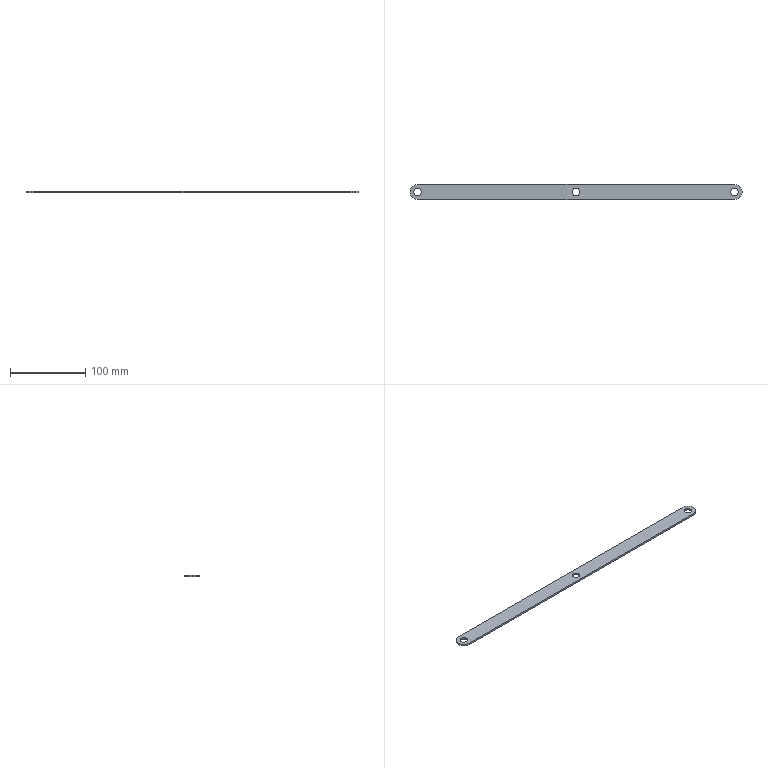Part | SolidWorks | features Extrusion 1 | 1 solid | 13 faces | box 440 x 20 x 2.5 mm | volume 21196 mm3 | cylinder 9 | plane 4 | commonest cylinder face diameters 10 x6 20 x3
STEP:
#1=CARTESIAN_POINT('',(-5.,0.,2.5));
#2=VERTEX_POINT('',#1);
#3=CARTESIAN_POINT('',(5.,0.,2.5));
#4=VERTEX_POINT('',#3);
#5=CARTESIAN_POINT('',(0.,0.,2.5));
#6=DIRECTION('',(0.,0.,1.));
#7=DIRECTION('',(1.,0.,0.));
#8=AXIS2_PLACEMENT_3D('',#5,#6,#7);
#9=CIRCLE('',#8,5.);
#10=EDGE_CURVE('',#2,#4,#9,.T.);
#11=ORIENTED_EDGE('',*,*,#10,.T.);
#12=CARTESIAN_POINT('',(5.,0.,0.));
#13=VERTEX_POINT('',#12);
#14=CARTESIAN_POINT('',(5.,0.,2.5));
#15=DIRECTION('',(0.,0.,-1.));
#16=VECTOR('',#15,1000.);
#17=LINE('',#14,#16);
#18=EDGE_CURVE('',#4,#13,#17,.T.);
#19=ORIENTED_EDGE('',*,*,#18,.T.);
#20=CARTESIAN_POINT('',(-5.,0.,0.));
#21=VERTEX_POINT('',#20);
#22=CARTESIAN_POINT('',(0.,0.,0.));
#23=DIRECTION('',(0.,0.,1.));
#24=DIRECTION('',(1.,0.,0.));
#25=AXIS2_PLACEMENT_3D('',#22,#23,#24);
#26=CIRCLE('',#25,5.);
#27=EDGE_CURVE('',#21,#13,#26,.T.);
#28=ORIENTED_EDGE('',*,*,#27,.F.);
#29=CARTESIAN_POINT('',(-5.,0.,2.5));
#30=DIRECTION('',(0.,0.,-1.));
#31=VECTOR('',#30,1000.);
#32=LINE('',#29,#31);
#33=EDGE_CURVE('',#2,#21,#32,.T.);
#34=ORIENTED_EDGE('',*,*,#33,.F.);
#35=EDGE_LOOP('',(#11,#19,#28,#34));
#36=FACE_OUTER_BOUND('',#35,.T.);
#37=CARTESIAN_POINT('',(0.,0.,2.5));
#38=DIRECTION('',(0.,0.,-1.));
#39=DIRECTION('',(-1.,0.,0.));
#40=AXIS2_PLACEMENT_3D('',#37,#38,#39);
#41=CYLINDRICAL_SURFACE('',#40,5.);
#42=ADVANCED_FACE('',(#36),#41,.F.);
#43=CARTESIAN_POINT('',(205.,0.,2.5));
#44=VERTEX_POINT('',#43);
#45=CARTESIAN_POINT('',(215.,0.,2.5));
#46=VERTEX_POINT('',#45);
#47=CARTESIAN_POINT('',(210.,0.,2.5));
#48=DIRECTION('',(0.,0.,1.));
#49=DIRECTION('',(1.,0.,0.));
#50=AXIS2_PLACEMENT_3D('',#47,#48,#49);
#51=CIRCLE('',#50,5.);
#52=EDGE_CURVE('',#44,#46,#51,.T.);
#53=ORIENTED_EDGE('',*,*,#52,.T.);
#54=CARTESIAN_POINT('',(215.,0.,0.));
#55=VERTEX_POINT('',#54);
#56=CARTESIAN_POINT('',(215.,0.,2.5));
#57=DIRECTION('',(0.,0.,-1.));
#58=VECTOR('',#57,1000.);
#59=LINE('',#56,#58);
#60=EDGE_CURVE('',#46,#55,#59,.T.);
#61=ORIENTED_EDGE('',*,*,#60,.T.);
#62=CARTESIAN_POINT('',(205.,0.,0.));
#63=VERTEX_POINT('',#62);
#64=CARTESIAN_POINT('',(210.,0.,0.));
#65=DIRECTION('',(0.,0.,1.));
#66=DIRECTION('',(1.,0.,0.));
#67=AXIS2_PLACEMENT_3D('',#64,#65,#66);
#68=CIRCLE('',#67,5.);
#69=EDGE_CURVE('',#63,#55,#68,.T.);
#70=ORIENTED_EDGE('',*,*,#69,.F.);
#71=CARTESIAN_POINT('',(205.,0.,2.5));
#72=DIRECTION('',(0.,0.,-1.));
#73=VECTOR('',#72,1000.);
#74=LINE('',#71,#73);
#75=EDGE_CURVE('',#44,#63,#74,.T.);
#76=ORIENTED_EDGE('',*,*,#75,.F.);
#77=EDGE_LOOP('',(#53,#61,#70,#76));
#78=FACE_OUTER_BOUND('',#77,.T.);
#79=CARTESIAN_POINT('',(210.,0.,2.5));
#80=DIRECTION('',(0.,0.,-1.));
#81=DIRECTION('',(-1.,0.,0.));
#82=AXIS2_PLACEMENT_3D('',#79,#80,#81);
#83=CYLINDRICAL_SURFACE('',#82,5.);
#84=ADVANCED_FACE('',(#78),#83,.F.);
#85=CARTESIAN_POINT('',(-215.,0.,2.5));
#86=VERTEX_POINT('',#85);
#87=CARTESIAN_POINT('',(-205.,0.,2.5));
#88=VERTEX_POINT('',#87);
#89=CARTESIAN_POINT('',(-210.,0.,2.5));
#90=DIRECTION('',(0.,0.,1.));
#91=DIRECTION('',(1.,0.,0.));
#92=AXIS2_PLACEMENT_3D('',#89,#90,#91);
#93=CIRCLE('',#92,5.);
#94=EDGE_CURVE('',#86,#88,#93,.T.);
#95=ORIENTED_EDGE('',*,*,#94,.T.);
#96=CARTESIAN_POINT('',(-205.,0.,0.));
#97=VERTEX_POINT('',#96);
#98=CARTESIAN_POINT('',(-205.,0.,2.5));
#99=DIRECTION('',(0.,0.,-1.));
#100=VECTOR('',#99,1000.);
#101=LINE('',#98,#100);
#102=EDGE_CURVE('',#88,#97,#101,.T.);
#103=ORIENTED_EDGE('',*,*,#102,.T.);
#104=CARTESIAN_POINT('',(-215.,0.,0.));
#105=VERTEX_POINT('',#104);
#106=CARTESIAN_POINT('',(-210.,0.,0.));
#107=DIRECTION('',(0.,0.,1.));
#108=DIRECTION('',(1.,0.,0.));
#109=AXIS2_PLACEMENT_3D('',#106,#107,#108);
#110=CIRCLE('',#109,5.);
#111=EDGE_CURVE('',#105,#97,#110,.T.);
#112=ORIENTED_EDGE('',*,*,#111,.F.);
#113=CARTESIAN_POINT('',(-215.,0.,2.5));
#114=DIRECTION('',(0.,0.,-1.));
#115=VECTOR('',#114,1000.);
#116=LINE('',#113,#115);
#117=EDGE_CURVE('',#86,#105,#116,.T.);
#118=ORIENTED_EDGE('',*,*,#117,.F.);
#119=EDGE_LOOP('',(#95,#103,#112,#118));
#120=FACE_OUTER_BOUND('',#119,.T.);
#121=CARTESIAN_POINT('',(-210.,0.,2.5));
#122=DIRECTION('',(0.,0.,-1.));
#123=DIRECTION('',(-1.,0.,0.));
#124=AXIS2_PLACEMENT_3D('',#121,#122,#123);
#125=CYLINDRICAL_SURFACE('',#124,5.);
#126=ADVANCED_FACE('',(#120),#125,.F.);
#127=CARTESIAN_POINT('',(-220.,0.,2.5));
#128=VERTEX_POINT('',#127);
#129=CARTESIAN_POINT('',(-210.,-10.,2.5));
#130=VERTEX_POINT('',#129);
#131=CARTESIAN_POINT('',(-210.,0.,2.5));
#132=DIRECTION('',(0.,0.,1.));
#133=DIRECTION('',(1.,0.,0.));
#134=AXIS2_PLACEMENT_3D('',#131,#132,#133);
#135=CIRCLE('',#134,10.);
#136=EDGE_CURVE('',#128,#130,#135,.T.);
#137=ORIENTED_EDGE('',*,*,#136,.F.);
#138=CARTESIAN_POINT('',(-220.,0.,0.));
#139=VERTEX_POINT('',#138);
#140=CARTESIAN_POINT('',(-220.,0.,2.5));
#141=DIRECTION('',(0.,0.,-1.));
#142=VECTOR('',#141,1000.);
#143=LINE('',#140,#142);
#144=EDGE_CURVE('',#128,#139,#143,.T.);
#145=ORIENTED_EDGE('',*,*,#144,.T.);
#146=CARTESIAN_POINT('',(-210.,-10.,0.));
#147=VERTEX_POINT('',#146);
#148=CARTESIAN_POINT('',(-210.,0.,0.));
#149=DIRECTION('',(0.,0.,1.));
#150=DIRECTION('',(1.,0.,0.));
#151=AXIS2_PLACEMENT_3D('',#148,#149,#150);
#152=CIRCLE('',#151,10.);
#153=EDGE_CURVE('',#139,#147,#152,.T.);
#154=ORIENTED_EDGE('',*,*,#153,.T.);
#155=CARTESIAN_POINT('',(-210.,-10.,2.5));
#156=DIRECTION('',(0.,0.,-1.));
#157=VECTOR('',#156,1000.);
#158=LINE('',#155,#157);
#159=EDGE_CURVE('',#130,#147,#158,.T.);
#160=ORIENTED_EDGE('',*,*,#159,.F.);
#161=EDGE_LOOP('',(#137,#145,#154,#160));
#162=FACE_OUTER_BOUND('',#161,.T.);
#163=CARTESIAN_POINT('',(-210.,0.,2.5));
#164=DIRECTION('',(0.,0.,-1.));
#165=DIRECTION('',(-1.,0.,0.));
#166=AXIS2_PLACEMENT_3D('',#163,#164,#165);
#167=CYLINDRICAL_SURFACE('',#166,10.);
#168=ADVANCED_FACE('',(#162),#167,.T.);
#169=ORIENTED_EDGE('',*,*,#52,.F.);
#170=CARTESIAN_POINT('',(210.,0.,2.5));
#171=DIRECTION('',(0.,0.,1.));
#172=DIRECTION('',(1.,0.,0.));
#173=AXIS2_PLACEMENT_3D('',#170,#171,#172);
#174=CIRCLE('',#173,5.);
#175=EDGE_CURVE('',#46,#44,#174,.T.);
#176=ORIENTED_EDGE('',*,*,#175,.F.);
#177=EDGE_LOOP('',(#169,#176));
#178=FACE_BOUND('',#177,.T.);
#179=CARTESIAN_POINT('',(-210.,10.,2.5));
#180=VERTEX_POINT('',#179);
#181=CARTESIAN_POINT('',(-210.,0.,2.5));
#182=DIRECTION('',(0.,0.,1.));
#183=DIRECTION('',(1.,0.,0.));
#184=AXIS2_PLACEMENT_3D('',#181,#182,#183);
#185=CIRCLE('',#184,10.);
#186=EDGE_CURVE('',#180,#128,#185,.T.);
#187=ORIENTED_EDGE('',*,*,#186,.T.);
#188=ORIENTED_EDGE('',*,*,#136,.T.);
#189=CARTESIAN_POINT('',(210.,-10.,2.5));
#190=VERTEX_POINT('',#189);
#191=CARTESIAN_POINT('',(-210.,-10.,2.5));
#192=DIRECTION('',(1.,0.,0.));
#193=VECTOR('',#192,1000.);
#194=LINE('',#191,#193);
#195=EDGE_CURVE('',#130,#190,#194,.T.);
#196=ORIENTED_EDGE('',*,*,#195,.T.);
#197=CARTESIAN_POINT('',(210.,10.,2.5));
#198=VERTEX_POINT('',#197);
#199=CARTESIAN_POINT('',(210.,0.,2.5));
#200=DIRECTION('',(0.,0.,1.));
#201=DIRECTION('',(1.,0.,0.));
#202=AXIS2_PLACEMENT_3D('',#199,#200,#201);
#203=CIRCLE('',#202,10.);
#204=EDGE_CURVE('',#190,#198,#203,.T.);
#205=ORIENTED_EDGE('',*,*,#204,.T.);
#206=CARTESIAN_POINT('',(-210.,10.,2.5));
#207=DIRECTION('',(-1.,0.,0.));
#208=VECTOR('',#207,1000.);
#209=LINE('',#206,#208);
#210=EDGE_CURVE('',#198,#180,#209,.T.);
#211=ORIENTED_EDGE('',*,*,#210,.T.);
#212=EDGE_LOOP('',(#187,#188,#196,#205,#211));
#213=FACE_OUTER_BOUND('',#212,.T.);
#214=ORIENTED_EDGE('',*,*,#94,.F.);
#215=CARTESIAN_POINT('',(-210.,0.,2.5));
#216=DIRECTION('',(0.,0.,1.));
#217=DIRECTION('',(1.,0.,0.));
#218=AXIS2_PLACEMENT_3D('',#215,#216,#217);
#219=CIRCLE('',#218,5.);
#220=EDGE_CURVE('',#88,#86,#219,.T.);
#221=ORIENTED_EDGE('',*,*,#220,.F.);
#222=EDGE_LOOP('',(#214,#221));
#223=FACE_BOUND('',#222,.T.);
#224=ORIENTED_EDGE('',*,*,#10,.F.);
#225=CARTESIAN_POINT('',(0.,0.,2.5));
#226=DIRECTION('',(0.,0.,1.));
#227=DIRECTION('',(1.,0.,0.));
#228=AXIS2_PLACEMENT_3D('',#225,#226,#227);
#229=CIRCLE('',#228,5.);
#230=EDGE_CURVE('',#4,#2,#229,.T.);
#231=ORIENTED_EDGE('',*,*,#230,.F.);
#232=EDGE_LOOP('',(#224,#231));
#233=FACE_BOUND('',#232,.T.);
#234=CARTESIAN_POINT('',(-210.,0.,2.5));
#235=DIRECTION('',(0.,0.,1.));
#236=DIRECTION('',(1.,0.,0.));
#237=AXIS2_PLACEMENT_3D('',#234,#235,#236);
#238=PLANE('',#237);
#239=ADVANCED_FACE('',(#178,#213,#223,#233),#238,.T.);
#240=CARTESIAN_POINT('',(-210.,10.,0.));
#241=VERTEX_POINT('',#240);
#242=CARTESIAN_POINT('',(-210.,0.,0.));
#243=DIRECTION('',(0.,0.,1.));
#244=DIRECTION('',(1.,0.,0.));
#245=AXIS2_PLACEMENT_3D('',#242,#243,#244);
#246=CIRCLE('',#245,10.);
#247=EDGE_CURVE('',#241,#139,#246,.T.);
#248=ORIENTED_EDGE('',*,*,#247,.F.);
#249=CARTESIAN_POINT('',(210.,10.,0.));
#250=VERTEX_POINT('',#249);
#251=CARTESIAN_POINT('',(-210.,10.,0.));
#252=DIRECTION('',(-1.,0.,0.));
#253=VECTOR('',#252,1000.);
#254=LINE('',#251,#253);
#255=EDGE_CURVE('',#250,#241,#254,.T.);
#256=ORIENTED_EDGE('',*,*,#255,.F.);
#257=CARTESIAN_POINT('',(210.,-10.,0.));
#258=VERTEX_POINT('',#257);
#259=CARTESIAN_POINT('',(210.,0.,0.));
#260=DIRECTION('',(0.,0.,1.));
#261=DIRECTION('',(1.,0.,0.));
#262=AXIS2_PLACEMENT_3D('',#259,#260,#261);
#263=CIRCLE('',#262,10.);
#264=EDGE_CURVE('',#258,#250,#263,.T.);
#265=ORIENTED_EDGE('',*,*,#264,.F.);
#266=CARTESIAN_POINT('',(-210.,-10.,0.));
#267=DIRECTION('',(1.,0.,0.));
#268=VECTOR('',#267,1000.);
#269=LINE('',#266,#268);
#270=EDGE_CURVE('',#147,#258,#269,.T.);
#271=ORIENTED_EDGE('',*,*,#270,.F.);
#272=ORIENTED_EDGE('',*,*,#153,.F.);
#273=EDGE_LOOP('',(#248,#256,#265,#271,#272));
#274=FACE_OUTER_BOUND('',#273,.T.);
#275=ORIENTED_EDGE('',*,*,#111,.T.);
#276=CARTESIAN_POINT('',(-210.,0.,0.));
#277=DIRECTION('',(0.,0.,1.));
#278=DIRECTION('',(1.,0.,0.));
#279=AXIS2_PLACEMENT_3D('',#276,#277,#278);
#280=CIRCLE('',#279,5.);
#281=EDGE_CURVE('',#97,#105,#280,.T.);
#282=ORIENTED_EDGE('',*,*,#281,.T.);
#283=EDGE_LOOP('',(#275,#282));
#284=FACE_BOUND('',#283,.T.);
#285=ORIENTED_EDGE('',*,*,#69,.T.);
#286=CARTESIAN_POINT('',(210.,0.,0.));
#287=DIRECTION('',(0.,0.,1.));
#288=DIRECTION('',(1.,0.,0.));
#289=AXIS2_PLACEMENT_3D('',#286,#287,#288);
#290=CIRCLE('',#289,5.);
#291=EDGE_CURVE('',#55,#63,#290,.T.);
#292=ORIENTED_EDGE('',*,*,#291,.T.);
#293=EDGE_LOOP('',(#285,#292));
#294=FACE_BOUND('',#293,.T.);
#295=ORIENTED_EDGE('',*,*,#27,.T.);
#296=CARTESIAN_POINT('',(0.,0.,0.));
#297=DIRECTION('',(0.,0.,1.));
#298=DIRECTION('',(1.,0.,0.));
#299=AXIS2_PLACEMENT_3D('',#296,#297,#298);
#300=CIRCLE('',#299,5.);
#301=EDGE_CURVE('',#13,#21,#300,.T.);
#302=ORIENTED_EDGE('',*,*,#301,.T.);
#303=EDGE_LOOP('',(#295,#302));
#304=FACE_BOUND('',#303,.T.);
#305=CARTESIAN_POINT('',(-210.,0.,0.));
#306=DIRECTION('',(0.,0.,1.));
#307=DIRECTION('',(1.,0.,0.));
#308=AXIS2_PLACEMENT_3D('',#305,#306,#307);
#309=PLANE('',#308);
#310=ADVANCED_FACE('',(#274,#284,#294,#304),#309,.F.);
#311=ORIENTED_EDGE('',*,*,#144,.F.);
#312=ORIENTED_EDGE('',*,*,#186,.F.);
#313=CARTESIAN_POINT('',(-210.,10.,2.5));
#314=DIRECTION('',(0.,0.,-1.));
#315=VECTOR('',#314,1000.);
#316=LINE('',#313,#315);
#317=EDGE_CURVE('',#180,#241,#316,.T.);
#318=ORIENTED_EDGE('',*,*,#317,.T.);
#319=ORIENTED_EDGE('',*,*,#247,.T.);
#320=EDGE_LOOP('',(#311,#312,#318,#319));
#321=FACE_OUTER_BOUND('',#320,.T.);
#322=CARTESIAN_POINT('',(-210.,0.,2.5));
#323=DIRECTION('',(0.,0.,-1.));
#324=DIRECTION('',(-1.,0.,0.));
#325=AXIS2_PLACEMENT_3D('',#322,#323,#324);
#326=CYLINDRICAL_SURFACE('',#325,10.);
#327=ADVANCED_FACE('',(#321),#326,.T.);
#328=ORIENTED_EDGE('',*,*,#270,.T.);
#329=CARTESIAN_POINT('',(210.,-10.,2.5));
#330=DIRECTION('',(0.,0.,-1.));
#331=VECTOR('',#330,1000.);
#332=LINE('',#329,#331);
#333=EDGE_CURVE('',#190,#258,#332,.T.);
#334=ORIENTED_EDGE('',*,*,#333,.F.);
#335=ORIENTED_EDGE('',*,*,#195,.F.);
#336=ORIENTED_EDGE('',*,*,#159,.T.);
#337=EDGE_LOOP('',(#328,#334,#335,#336));
#338=FACE_OUTER_BOUND('',#337,.T.);
#339=CARTESIAN_POINT('',(-210.,-10.,2.5));
#340=DIRECTION('',(0.,1.,0.));
#341=DIRECTION('',(0.,0.,1.));
#342=AXIS2_PLACEMENT_3D('',#339,#340,#341);
#343=PLANE('',#342);
#344=ADVANCED_FACE('',(#338),#343,.F.);
#345=ORIENTED_EDGE('',*,*,#264,.T.);
#346=CARTESIAN_POINT('',(210.,10.,2.5));
#347=DIRECTION('',(0.,0.,-1.));
#348=VECTOR('',#347,1000.);
#349=LINE('',#346,#348);
#350=EDGE_CURVE('',#198,#250,#349,.T.);
#351=ORIENTED_EDGE('',*,*,#350,.F.);
#352=ORIENTED_EDGE('',*,*,#204,.F.);
#353=ORIENTED_EDGE('',*,*,#333,.T.);
#354=EDGE_LOOP('',(#345,#351,#352,#353));
#355=FACE_OUTER_BOUND('',#354,.T.);
#356=CARTESIAN_POINT('',(210.,0.,2.5));
#357=DIRECTION('',(0.,0.,-1.));
#358=DIRECTION('',(-1.,0.,0.));
#359=AXIS2_PLACEMENT_3D('',#356,#357,#358);
#360=CYLINDRICAL_SURFACE('',#359,10.);
#361=ADVANCED_FACE('',(#355),#360,.T.);
#362=ORIENTED_EDGE('',*,*,#255,.T.);
#363=ORIENTED_EDGE('',*,*,#317,.F.);
#364=ORIENTED_EDGE('',*,*,#210,.F.);
#365=ORIENTED_EDGE('',*,*,#350,.T.);
#366=EDGE_LOOP('',(#362,#363,#364,#365));
#367=FACE_OUTER_BOUND('',#366,.T.);
#368=CARTESIAN_POINT('',(-210.,10.,2.5));
#369=DIRECTION('',(0.,-1.,0.));
#370=DIRECTION('',(0.,0.,-1.));
#371=AXIS2_PLACEMENT_3D('',#368,#369,#370);
#372=PLANE('',#371);
#373=ADVANCED_FACE('',(#367),#372,.F.);
#374=ORIENTED_EDGE('',*,*,#102,.F.);
#375=ORIENTED_EDGE('',*,*,#220,.T.);
#376=ORIENTED_EDGE('',*,*,#117,.T.);
#377=ORIENTED_EDGE('',*,*,#281,.F.);
#378=EDGE_LOOP('',(#374,#375,#376,#377));
#379=FACE_OUTER_BOUND('',#378,.T.);
#380=CARTESIAN_POINT('',(-210.,0.,2.5));
#381=DIRECTION('',(0.,0.,-1.));
#382=DIRECTION('',(-1.,0.,0.));
#383=AXIS2_PLACEMENT_3D('',#380,#381,#382);
#384=CYLINDRICAL_SURFACE('',#383,5.);
#385=ADVANCED_FACE('',(#379),#384,.F.);
#386=ORIENTED_EDGE('',*,*,#60,.F.);
#387=ORIENTED_EDGE('',*,*,#175,.T.);
#388=ORIENTED_EDGE('',*,*,#75,.T.);
#389=ORIENTED_EDGE('',*,*,#291,.F.);
#390=EDGE_LOOP('',(#386,#387,#388,#389));
#391=FACE_OUTER_BOUND('',#390,.T.);
#392=CARTESIAN_POINT('',(210.,0.,2.5));
#393=DIRECTION('',(0.,0.,-1.));
#394=DIRECTION('',(-1.,0.,0.));
#395=AXIS2_PLACEMENT_3D('',#392,#393,#394);
#396=CYLINDRICAL_SURFACE('',#395,5.);
#397=ADVANCED_FACE('',(#391),#396,.F.);
#398=ORIENTED_EDGE('',*,*,#18,.F.);
#399=ORIENTED_EDGE('',*,*,#230,.T.);
#400=ORIENTED_EDGE('',*,*,#33,.T.);
#401=ORIENTED_EDGE('',*,*,#301,.F.);
#402=EDGE_LOOP('',(#398,#399,#400,#401));
#403=FACE_OUTER_BOUND('',#402,.T.);
#404=CARTESIAN_POINT('',(0.,0.,2.5));
#405=DIRECTION('',(0.,0.,-1.));
#406=DIRECTION('',(-1.,0.,0.));
#407=AXIS2_PLACEMENT_3D('',#404,#405,#406);
#408=CYLINDRICAL_SURFACE('',#407,5.);
#409=ADVANCED_FACE('',(#403),#408,.F.);
#410=CLOSED_SHELL('',(#42,#84,#126,#168,#239,#310,#327,#344,#361,#373,#385,#397,#409));
#411=MANIFOLD_SOLID_BREP('',#410);
#412=CARTESIAN_POINT('',(0.,0.,0.));
#413=DIRECTION('',(0.,0.,1.));
#414=DIRECTION('',(1.,0.,0.));
#415=AXIS2_PLACEMENT_3D('',#412,#413,#414);
#416=(LENGTH_UNIT()NAMED_UNIT(*)SI_UNIT(.MILLI.,.METRE.));
#417=UNCERTAINTY_MEASURE_WITH_UNIT(LENGTH_MEASURE(0.00001),#416,'','');
#418=(NAMED_UNIT(*)PLANE_ANGLE_UNIT()SI_UNIT($,.RADIAN.));
#419=(NAMED_UNIT(*)SI_UNIT($,.STERADIAN.)SOLID_ANGLE_UNIT());
#420=(GEOMETRIC_REPRESENTATION_CONTEXT(3)GLOBAL_UNCERTAINTY_ASSIGNED_CONTEXT((#417))GLOBAL_UNIT_ASSIGNED_CONTEXT((#416,#418,#419))REPRESENTATION_CONTEXT('',''));
#421=ADVANCED_BREP_SHAPE_REPRESENTATION('',(#411,#415),#420);